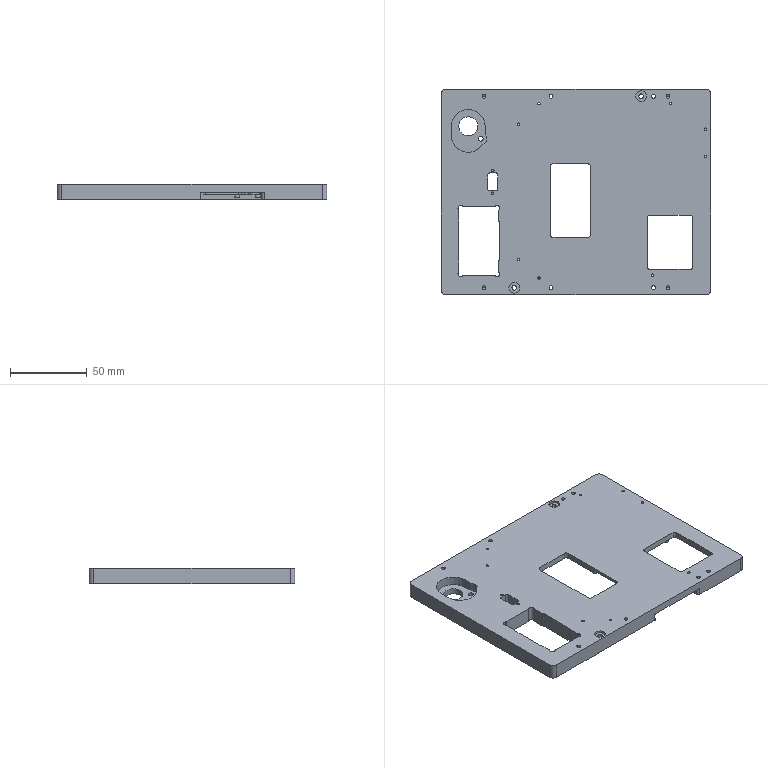NC program | NX | posted with a generic post | part box 176 x 134 x 10 mm
Lines 1 to 123 of 8914:
N10 G17 G21 G94 G90
(FLOOR_WALL_COPY , TOOL : D63)
N12 T03 M6
N14 G54
N16 G17 G0 G90 X-126.5 Y70.999 S6500 M3
N18 G43 Z30. H3
N20 Z3.
N22 G94 G1 Z0. F1250.
N24 X-123.5
N26 X123.5
N28 Y32.066
N30 X-123.5
N32 Y-6.867
N34 X123.5
N36 Y-45.8
N38 X-123.5
N40 X-126.5
N42 Z3.
N44 G0 Z30.
N46 M5
(DRILLING_COPY_1 , TOOL : D6A45)
N48 T01 M6
N50 G54
N52 G17 G0 G90 X60. Y-62.5 S5000 M3
N54 G43 Z30. H1
N56 G94 G81 G98 Z-0.5 F250. R3.
N58 X50.599
N60 X49.84 Y-54.316
N62 X-16.297 Y-62.5
N64 X-24.201 Y-56.204
N66 X-37.5 Y-44.
N68 X-40.297 Y-62.5
N70 X-51.552 Y-53.439
N72 X-60. Y-62.5
N74 X-75.302 Y-53.439
N76 Y-10.539
N78 X-51.552
N80 X-54.332 Y-0.797
N82 X-54.317 Y14.043
N84 X-62.16 Y34.784
N86 X-70.284 Y42.924
N88 X-60. Y62.5
N90 X-37.576 Y44.253
N92 X-24.201 Y57.656
N94 X-16.297 Y62.5
N96 X42.499
N98 X50.599
N100 X60.
N102 X61.81 Y57.575
N104 X84.5 Y41.
N106 Y23.
N108 G80
N110 G0 X84.5 Y23. Z30.
N112 M5
(DRILLING_COPY_1_COPY_1 , TOOL : 3.5ZT)
N114 T13 M6
N116 G54
N118 G17 G0 G90 X-51.552 Y-53.439 S2000 M3
N120 G43 Z30. H13
N122 G94 G83 G98 Z-12.552 F150. Q2. R3.
N124 X-75.302
N126 Y-10.539
N128 X-51.552
N130 G80
N132 G0 X-51.552 Y-10.539 Z30.
N134 M5
(DRILLING_COPY_1_COPY_COPY , TOOL : 2.5ZT)
N136 T12 M6
N138 G54
N140 G17 G0 G90 X60. Y62.5 S2000 M3
N142 G43 Z30. H12
N144 G94 G83 G98 Z-7.751 F150. Q2. R3.
N146 X50.599 Z-12.051
N148 X-16.297
N150 X-60. Z-7.751
N152 Y-62.5
N154 X-16.297 Z-12.051
N156 X50.599
N158 X60. Z-7.751
N160 G80
N162 G0 X60. Y-62.5 Z30.
N164 M5
(DRILLING_COPY_1_COPY , TOOL : 1.6ZT)
N166 T20 M6
N168 G54
N170 G17 G0 G90 X61.81 Y57.575 S2000 M3
N172 G43 Z30. H20
N174 G94 G83 G98 Z-8.881 F100. Q2. R3.
N176 X84.5 Y41. Z-6.981
N178 Y23.
N180 X49.84 Y-54.316 Z-8.881
N182 X-24.201 Y-56.204
N184 X-37.5 Y-44.
N186 X-54.332 Y-0.797 Z-7.681
N188 X-54.317 Y14.043
N190 X-37.576 Y44.253 Z-8.881
N192 X-24.201 Y57.656
N194 G80
N196 G0 X-24.201 Y57.656 Z30.
N198 M5
(DRILLING_COPY_1_COPY_COPY_COPY , TOOL : 3.2ZT)
N200 T23 M6
N202 G54
N204 G17 G0 G90 X-62.16 Y34.784 S2000 M3
N206 G43 Z30. H23
N208 G94 G83 G98 Z-12.461 F150. Q2. R3.
N210 G80
N212 G0 X-62.16 Y34.784 Z30.
N214 M5